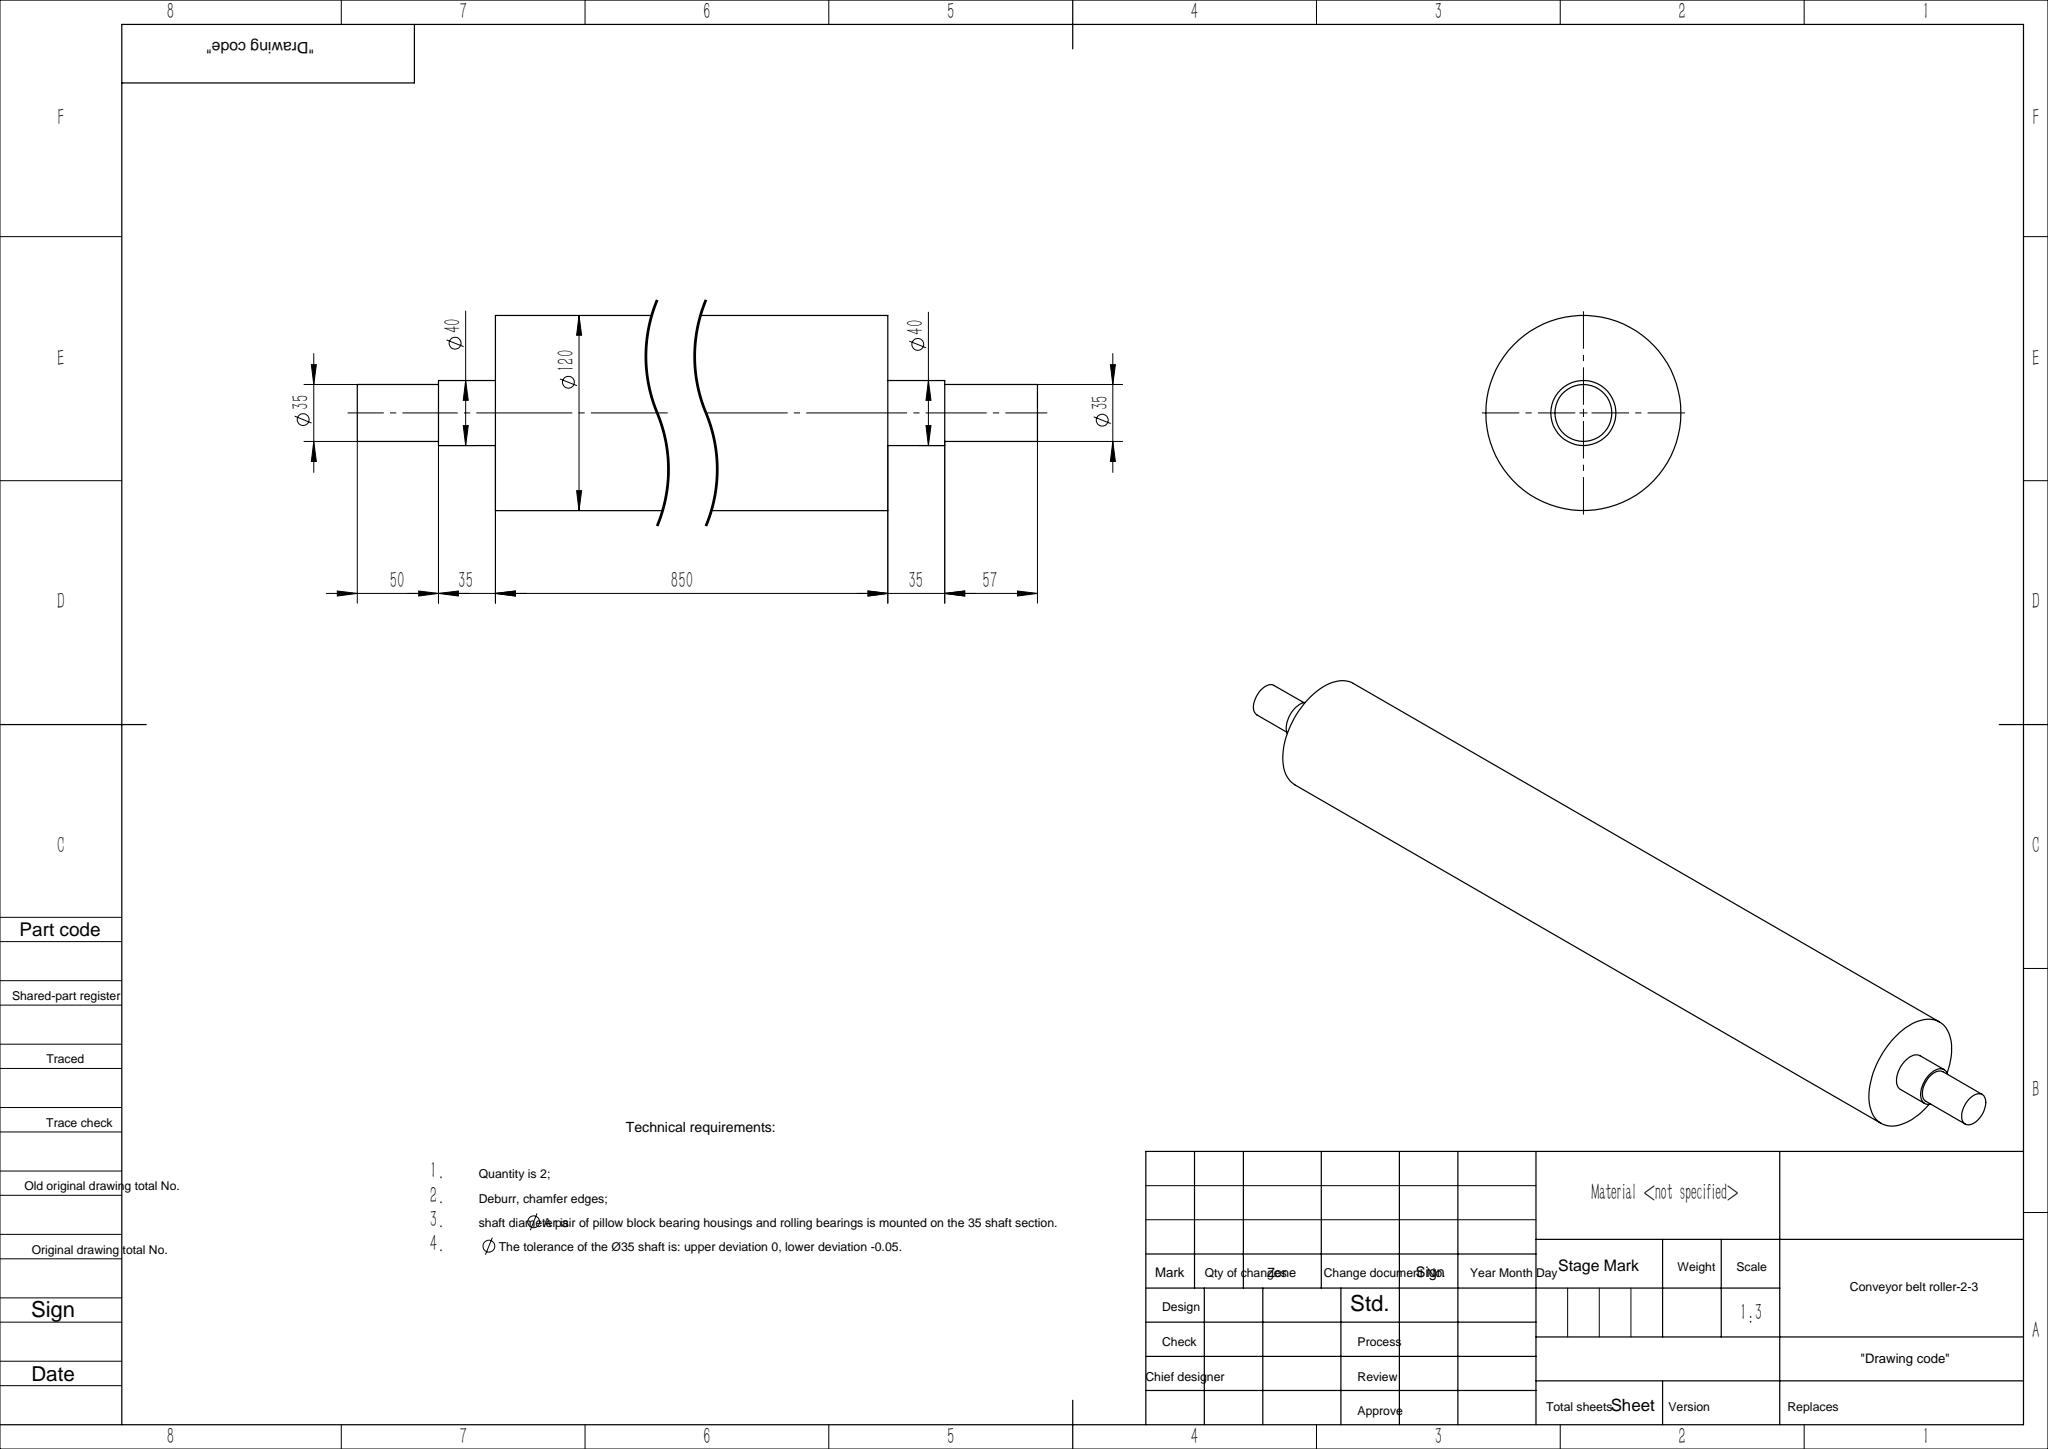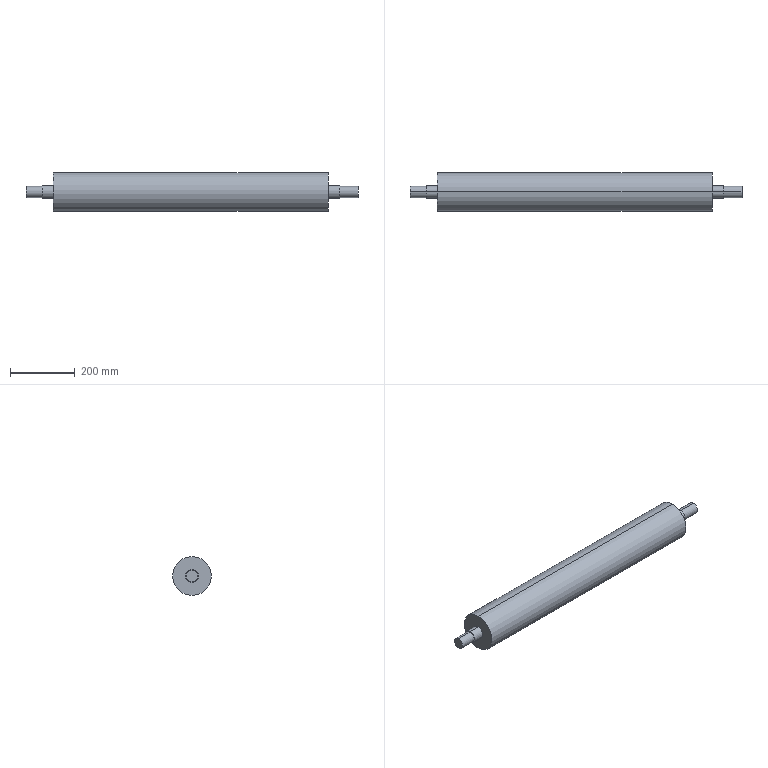Part | SolidWorks | features Revolution 1 | 1 solid | 16 faces | box 1027 x 120 x 120 mm | volume 9804184 mm3 | cylinder 10 | plane 6 | commonest cylinder face diameters 35 x4 40 x4 120 x2
STEP:
#1=CARTESIAN_POINT('',(970.,0.,-17.5));
#2=VERTEX_POINT('',#1);
#3=CARTESIAN_POINT('',(970.,0.,17.5));
#4=VERTEX_POINT('',#3);
#5=CARTESIAN_POINT('',(970.,0.,0.));
#6=DIRECTION('',(1.,0.,0.));
#7=DIRECTION('',(0.,0.,-1.));
#8=AXIS2_PLACEMENT_3D('',#5,#6,#7);
#9=CIRCLE('',#8,17.5);
#10=EDGE_CURVE('',#2,#4,#9,.T.);
#11=ORIENTED_EDGE('',*,*,#10,.T.);
#12=CARTESIAN_POINT('',(1027.,0.,17.5));
#13=VERTEX_POINT('',#12);
#14=CARTESIAN_POINT('',(1027.,0.,17.5));
#15=DIRECTION('',(1.,0.,0.));
#16=VECTOR('',#15,1000.);
#17=LINE('',#14,#16);
#18=EDGE_CURVE('',#4,#13,#17,.T.);
#19=ORIENTED_EDGE('',*,*,#18,.T.);
#20=CARTESIAN_POINT('',(1027.,0.,-17.5));
#21=VERTEX_POINT('',#20);
#22=CARTESIAN_POINT('',(1027.,0.,0.));
#23=DIRECTION('',(1.,0.,0.));
#24=DIRECTION('',(0.,0.,-1.));
#25=AXIS2_PLACEMENT_3D('',#22,#23,#24);
#26=CIRCLE('',#25,17.5);
#27=EDGE_CURVE('',#21,#13,#26,.T.);
#28=ORIENTED_EDGE('',*,*,#27,.F.);
#29=CARTESIAN_POINT('',(1027.,0.,-17.5));
#30=DIRECTION('',(1.,0.,0.));
#31=VECTOR('',#30,1000.);
#32=LINE('',#29,#31);
#33=EDGE_CURVE('',#2,#21,#32,.T.);
#34=ORIENTED_EDGE('',*,*,#33,.F.);
#35=EDGE_LOOP('',(#11,#19,#28,#34));
#36=FACE_OUTER_BOUND('',#35,.T.);
#37=CARTESIAN_POINT('',(1027.,0.,0.));
#38=DIRECTION('',(1.,0.,0.));
#39=DIRECTION('',(0.,0.,-1.));
#40=AXIS2_PLACEMENT_3D('',#37,#38,#39);
#41=CYLINDRICAL_SURFACE('',#40,17.5);
#42=ADVANCED_FACE('',(#36),#41,.T.);
#43=CARTESIAN_POINT('',(935.,0.,-20.));
#44=VERTEX_POINT('',#43);
#45=CARTESIAN_POINT('',(935.,0.,20.));
#46=VERTEX_POINT('',#45);
#47=CARTESIAN_POINT('',(935.,0.,0.));
#48=DIRECTION('',(1.,0.,0.));
#49=DIRECTION('',(0.,0.,-1.));
#50=AXIS2_PLACEMENT_3D('',#47,#48,#49);
#51=CIRCLE('',#50,20.);
#52=EDGE_CURVE('',#44,#46,#51,.T.);
#53=ORIENTED_EDGE('',*,*,#52,.T.);
#54=CARTESIAN_POINT('',(970.,0.,20.));
#55=VERTEX_POINT('',#54);
#56=CARTESIAN_POINT('',(1027.,0.,20.));
#57=DIRECTION('',(1.,0.,0.));
#58=VECTOR('',#57,1000.);
#59=LINE('',#56,#58);
#60=EDGE_CURVE('',#46,#55,#59,.T.);
#61=ORIENTED_EDGE('',*,*,#60,.T.);
#62=CARTESIAN_POINT('',(970.,0.,-20.));
#63=VERTEX_POINT('',#62);
#64=CARTESIAN_POINT('',(970.,0.,0.));
#65=DIRECTION('',(1.,0.,0.));
#66=DIRECTION('',(0.,0.,-1.));
#67=AXIS2_PLACEMENT_3D('',#64,#65,#66);
#68=CIRCLE('',#67,20.);
#69=EDGE_CURVE('',#63,#55,#68,.T.);
#70=ORIENTED_EDGE('',*,*,#69,.F.);
#71=CARTESIAN_POINT('',(1027.,0.,-20.));
#72=DIRECTION('',(1.,0.,0.));
#73=VECTOR('',#72,1000.);
#74=LINE('',#71,#73);
#75=EDGE_CURVE('',#44,#63,#74,.T.);
#76=ORIENTED_EDGE('',*,*,#75,.F.);
#77=EDGE_LOOP('',(#53,#61,#70,#76));
#78=FACE_OUTER_BOUND('',#77,.T.);
#79=CARTESIAN_POINT('',(1027.,0.,0.));
#80=DIRECTION('',(1.,0.,0.));
#81=DIRECTION('',(0.,0.,-1.));
#82=AXIS2_PLACEMENT_3D('',#79,#80,#81);
#83=CYLINDRICAL_SURFACE('',#82,20.);
#84=ADVANCED_FACE('',(#78),#83,.T.);
#85=CARTESIAN_POINT('',(85.,0.,-60.));
#86=VERTEX_POINT('',#85);
#87=CARTESIAN_POINT('',(85.,0.,60.));
#88=VERTEX_POINT('',#87);
#89=CARTESIAN_POINT('',(85.,0.,0.));
#90=DIRECTION('',(1.,0.,0.));
#91=DIRECTION('',(0.,0.,-1.));
#92=AXIS2_PLACEMENT_3D('',#89,#90,#91);
#93=CIRCLE('',#92,60.);
#94=EDGE_CURVE('',#86,#88,#93,.T.);
#95=ORIENTED_EDGE('',*,*,#94,.T.);
#96=CARTESIAN_POINT('',(935.,0.,60.));
#97=VERTEX_POINT('',#96);
#98=CARTESIAN_POINT('',(1027.,0.,60.));
#99=DIRECTION('',(1.,0.,0.));
#100=VECTOR('',#99,1000.);
#101=LINE('',#98,#100);
#102=EDGE_CURVE('',#88,#97,#101,.T.);
#103=ORIENTED_EDGE('',*,*,#102,.T.);
#104=CARTESIAN_POINT('',(935.,0.,-60.));
#105=VERTEX_POINT('',#104);
#106=CARTESIAN_POINT('',(935.,0.,0.));
#107=DIRECTION('',(1.,0.,0.));
#108=DIRECTION('',(0.,0.,-1.));
#109=AXIS2_PLACEMENT_3D('',#106,#107,#108);
#110=CIRCLE('',#109,60.);
#111=EDGE_CURVE('',#105,#97,#110,.T.);
#112=ORIENTED_EDGE('',*,*,#111,.F.);
#113=CARTESIAN_POINT('',(1027.,0.,-60.));
#114=DIRECTION('',(1.,0.,0.));
#115=VECTOR('',#114,1000.);
#116=LINE('',#113,#115);
#117=EDGE_CURVE('',#86,#105,#116,.T.);
#118=ORIENTED_EDGE('',*,*,#117,.F.);
#119=EDGE_LOOP('',(#95,#103,#112,#118));
#120=FACE_OUTER_BOUND('',#119,.T.);
#121=CARTESIAN_POINT('',(1027.,0.,0.));
#122=DIRECTION('',(1.,0.,0.));
#123=DIRECTION('',(0.,0.,-1.));
#124=AXIS2_PLACEMENT_3D('',#121,#122,#123);
#125=CYLINDRICAL_SURFACE('',#124,60.);
#126=ADVANCED_FACE('',(#120),#125,.T.);
#127=CARTESIAN_POINT('',(50.,0.,-20.));
#128=VERTEX_POINT('',#127);
#129=CARTESIAN_POINT('',(50.,0.,20.));
#130=VERTEX_POINT('',#129);
#131=CARTESIAN_POINT('',(50.,0.,0.));
#132=DIRECTION('',(1.,0.,0.));
#133=DIRECTION('',(0.,0.,-1.));
#134=AXIS2_PLACEMENT_3D('',#131,#132,#133);
#135=CIRCLE('',#134,20.);
#136=EDGE_CURVE('',#128,#130,#135,.T.);
#137=ORIENTED_EDGE('',*,*,#136,.T.);
#138=CARTESIAN_POINT('',(85.,0.,20.));
#139=VERTEX_POINT('',#138);
#140=CARTESIAN_POINT('',(1027.,0.,20.));
#141=DIRECTION('',(1.,0.,0.));
#142=VECTOR('',#141,1000.);
#143=LINE('',#140,#142);
#144=EDGE_CURVE('',#130,#139,#143,.T.);
#145=ORIENTED_EDGE('',*,*,#144,.T.);
#146=CARTESIAN_POINT('',(85.,0.,-20.));
#147=VERTEX_POINT('',#146);
#148=CARTESIAN_POINT('',(85.,0.,0.));
#149=DIRECTION('',(1.,0.,0.));
#150=DIRECTION('',(0.,0.,-1.));
#151=AXIS2_PLACEMENT_3D('',#148,#149,#150);
#152=CIRCLE('',#151,20.);
#153=EDGE_CURVE('',#147,#139,#152,.T.);
#154=ORIENTED_EDGE('',*,*,#153,.F.);
#155=CARTESIAN_POINT('',(1027.,0.,-20.));
#156=DIRECTION('',(1.,0.,0.));
#157=VECTOR('',#156,1000.);
#158=LINE('',#155,#157);
#159=EDGE_CURVE('',#128,#147,#158,.T.);
#160=ORIENTED_EDGE('',*,*,#159,.F.);
#161=EDGE_LOOP('',(#137,#145,#154,#160));
#162=FACE_OUTER_BOUND('',#161,.T.);
#163=CARTESIAN_POINT('',(1027.,0.,0.));
#164=DIRECTION('',(1.,0.,0.));
#165=DIRECTION('',(0.,0.,-1.));
#166=AXIS2_PLACEMENT_3D('',#163,#164,#165);
#167=CYLINDRICAL_SURFACE('',#166,20.);
#168=ADVANCED_FACE('',(#162),#167,.T.);
#169=CARTESIAN_POINT('',(0.,0.,-17.5));
#170=VERTEX_POINT('',#169);
#171=CARTESIAN_POINT('',(0.,0.,17.5));
#172=VERTEX_POINT('',#171);
#173=CARTESIAN_POINT('',(0.,0.,0.));
#174=DIRECTION('',(1.,0.,0.));
#175=DIRECTION('',(0.,0.,-1.));
#176=AXIS2_PLACEMENT_3D('',#173,#174,#175);
#177=CIRCLE('',#176,17.5);
#178=EDGE_CURVE('',#170,#172,#177,.T.);
#179=ORIENTED_EDGE('',*,*,#178,.T.);
#180=CARTESIAN_POINT('',(50.,0.,17.5));
#181=VERTEX_POINT('',#180);
#182=CARTESIAN_POINT('',(1027.,0.,17.5));
#183=DIRECTION('',(1.,0.,0.));
#184=VECTOR('',#183,1000.);
#185=LINE('',#182,#184);
#186=EDGE_CURVE('',#172,#181,#185,.T.);
#187=ORIENTED_EDGE('',*,*,#186,.T.);
#188=CARTESIAN_POINT('',(50.,0.,-17.5));
#189=VERTEX_POINT('',#188);
#190=CARTESIAN_POINT('',(50.,0.,0.));
#191=DIRECTION('',(1.,0.,0.));
#192=DIRECTION('',(0.,0.,-1.));
#193=AXIS2_PLACEMENT_3D('',#190,#191,#192);
#194=CIRCLE('',#193,17.5);
#195=EDGE_CURVE('',#189,#181,#194,.T.);
#196=ORIENTED_EDGE('',*,*,#195,.F.);
#197=CARTESIAN_POINT('',(1027.,0.,-17.5));
#198=DIRECTION('',(1.,0.,0.));
#199=VECTOR('',#198,1000.);
#200=LINE('',#197,#199);
#201=EDGE_CURVE('',#170,#189,#200,.T.);
#202=ORIENTED_EDGE('',*,*,#201,.F.);
#203=EDGE_LOOP('',(#179,#187,#196,#202));
#204=FACE_OUTER_BOUND('',#203,.T.);
#205=CARTESIAN_POINT('',(1027.,0.,0.));
#206=DIRECTION('',(1.,0.,0.));
#207=DIRECTION('',(0.,0.,-1.));
#208=AXIS2_PLACEMENT_3D('',#205,#206,#207);
#209=CYLINDRICAL_SURFACE('',#208,17.5);
#210=ADVANCED_FACE('',(#204),#209,.T.);
#211=ORIENTED_EDGE('',*,*,#178,.F.);
#212=CARTESIAN_POINT('',(0.,0.,0.));
#213=DIRECTION('',(1.,0.,0.));
#214=DIRECTION('',(0.,0.,-1.));
#215=AXIS2_PLACEMENT_3D('',#212,#213,#214);
#216=CIRCLE('',#215,17.5);
#217=EDGE_CURVE('',#172,#170,#216,.T.);
#218=ORIENTED_EDGE('',*,*,#217,.F.);
#219=EDGE_LOOP('',(#211,#218));
#220=FACE_OUTER_BOUND('',#219,.T.);
#221=CARTESIAN_POINT('',(0.,0.,0.));
#222=DIRECTION('',(-1.,0.,0.));
#223=DIRECTION('',(0.,0.,1.));
#224=AXIS2_PLACEMENT_3D('',#221,#222,#223);
#225=PLANE('',#224);
#226=ADVANCED_FACE('',(#220),#225,.T.);
#227=ORIENTED_EDGE('',*,*,#186,.F.);
#228=ORIENTED_EDGE('',*,*,#217,.T.);
#229=ORIENTED_EDGE('',*,*,#201,.T.);
#230=CARTESIAN_POINT('',(50.,0.,0.));
#231=DIRECTION('',(1.,0.,0.));
#232=DIRECTION('',(0.,0.,-1.));
#233=AXIS2_PLACEMENT_3D('',#230,#231,#232);
#234=CIRCLE('',#233,17.5);
#235=EDGE_CURVE('',#181,#189,#234,.T.);
#236=ORIENTED_EDGE('',*,*,#235,.F.);
#237=EDGE_LOOP('',(#227,#228,#229,#236));
#238=FACE_OUTER_BOUND('',#237,.T.);
#239=CARTESIAN_POINT('',(1027.,0.,0.));
#240=DIRECTION('',(1.,0.,0.));
#241=DIRECTION('',(0.,0.,-1.));
#242=AXIS2_PLACEMENT_3D('',#239,#240,#241);
#243=CYLINDRICAL_SURFACE('',#242,17.5);
#244=ADVANCED_FACE('',(#238),#243,.T.);
#245=ORIENTED_EDGE('',*,*,#195,.T.);
#246=ORIENTED_EDGE('',*,*,#235,.T.);
#247=EDGE_LOOP('',(#245,#246));
#248=FACE_BOUND('',#247,.T.);
#249=ORIENTED_EDGE('',*,*,#136,.F.);
#250=CARTESIAN_POINT('',(50.,0.,0.));
#251=DIRECTION('',(1.,0.,0.));
#252=DIRECTION('',(0.,0.,-1.));
#253=AXIS2_PLACEMENT_3D('',#250,#251,#252);
#254=CIRCLE('',#253,20.);
#255=EDGE_CURVE('',#130,#128,#254,.T.);
#256=ORIENTED_EDGE('',*,*,#255,.F.);
#257=EDGE_LOOP('',(#249,#256));
#258=FACE_OUTER_BOUND('',#257,.T.);
#259=CARTESIAN_POINT('',(50.,17.5,0.));
#260=DIRECTION('',(-1.,0.,0.));
#261=DIRECTION('',(0.,0.,1.));
#262=AXIS2_PLACEMENT_3D('',#259,#260,#261);
#263=PLANE('',#262);
#264=ADVANCED_FACE('',(#248,#258),#263,.T.);
#265=ORIENTED_EDGE('',*,*,#144,.F.);
#266=ORIENTED_EDGE('',*,*,#255,.T.);
#267=ORIENTED_EDGE('',*,*,#159,.T.);
#268=CARTESIAN_POINT('',(85.,0.,0.));
#269=DIRECTION('',(1.,0.,0.));
#270=DIRECTION('',(0.,0.,-1.));
#271=AXIS2_PLACEMENT_3D('',#268,#269,#270);
#272=CIRCLE('',#271,20.);
#273=EDGE_CURVE('',#139,#147,#272,.T.);
#274=ORIENTED_EDGE('',*,*,#273,.F.);
#275=EDGE_LOOP('',(#265,#266,#267,#274));
#276=FACE_OUTER_BOUND('',#275,.T.);
#277=CARTESIAN_POINT('',(1027.,0.,0.));
#278=DIRECTION('',(1.,0.,0.));
#279=DIRECTION('',(0.,0.,-1.));
#280=AXIS2_PLACEMENT_3D('',#277,#278,#279);
#281=CYLINDRICAL_SURFACE('',#280,20.);
#282=ADVANCED_FACE('',(#276),#281,.T.);
#283=ORIENTED_EDGE('',*,*,#153,.T.);
#284=ORIENTED_EDGE('',*,*,#273,.T.);
#285=EDGE_LOOP('',(#283,#284));
#286=FACE_BOUND('',#285,.T.);
#287=ORIENTED_EDGE('',*,*,#94,.F.);
#288=CARTESIAN_POINT('',(85.,0.,0.));
#289=DIRECTION('',(1.,0.,0.));
#290=DIRECTION('',(0.,0.,-1.));
#291=AXIS2_PLACEMENT_3D('',#288,#289,#290);
#292=CIRCLE('',#291,60.);
#293=EDGE_CURVE('',#88,#86,#292,.T.);
#294=ORIENTED_EDGE('',*,*,#293,.F.);
#295=EDGE_LOOP('',(#287,#294));
#296=FACE_OUTER_BOUND('',#295,.T.);
#297=CARTESIAN_POINT('',(85.,20.,0.));
#298=DIRECTION('',(-1.,0.,0.));
#299=DIRECTION('',(0.,0.,1.));
#300=AXIS2_PLACEMENT_3D('',#297,#298,#299);
#301=PLANE('',#300);
#302=ADVANCED_FACE('',(#286,#296),#301,.T.);
#303=ORIENTED_EDGE('',*,*,#102,.F.);
#304=ORIENTED_EDGE('',*,*,#293,.T.);
#305=ORIENTED_EDGE('',*,*,#117,.T.);
#306=CARTESIAN_POINT('',(935.,0.,0.));
#307=DIRECTION('',(1.,0.,0.));
#308=DIRECTION('',(0.,0.,-1.));
#309=AXIS2_PLACEMENT_3D('',#306,#307,#308);
#310=CIRCLE('',#309,60.);
#311=EDGE_CURVE('',#97,#105,#310,.T.);
#312=ORIENTED_EDGE('',*,*,#311,.F.);
#313=EDGE_LOOP('',(#303,#304,#305,#312));
#314=FACE_OUTER_BOUND('',#313,.T.);
#315=CARTESIAN_POINT('',(1027.,0.,0.));
#316=DIRECTION('',(1.,0.,0.));
#317=DIRECTION('',(0.,0.,-1.));
#318=AXIS2_PLACEMENT_3D('',#315,#316,#317);
#319=CYLINDRICAL_SURFACE('',#318,60.);
#320=ADVANCED_FACE('',(#314),#319,.T.);
#321=ORIENTED_EDGE('',*,*,#111,.T.);
#322=ORIENTED_EDGE('',*,*,#311,.T.);
#323=EDGE_LOOP('',(#321,#322));
#324=FACE_OUTER_BOUND('',#323,.T.);
#325=ORIENTED_EDGE('',*,*,#52,.F.);
#326=CARTESIAN_POINT('',(935.,0.,0.));
#327=DIRECTION('',(1.,0.,0.));
#328=DIRECTION('',(0.,0.,-1.));
#329=AXIS2_PLACEMENT_3D('',#326,#327,#328);
#330=CIRCLE('',#329,20.);
#331=EDGE_CURVE('',#46,#44,#330,.T.);
#332=ORIENTED_EDGE('',*,*,#331,.F.);
#333=EDGE_LOOP('',(#325,#332));
#334=FACE_BOUND('',#333,.T.);
#335=CARTESIAN_POINT('',(935.,60.,0.));
#336=DIRECTION('',(1.,0.,0.));
#337=DIRECTION('',(0.,0.,-1.));
#338=AXIS2_PLACEMENT_3D('',#335,#336,#337);
#339=PLANE('',#338);
#340=ADVANCED_FACE('',(#324,#334),#339,.T.);
#341=ORIENTED_EDGE('',*,*,#60,.F.);
#342=ORIENTED_EDGE('',*,*,#331,.T.);
#343=ORIENTED_EDGE('',*,*,#75,.T.);
#344=CARTESIAN_POINT('',(970.,0.,0.));
#345=DIRECTION('',(1.,0.,0.));
#346=DIRECTION('',(0.,0.,-1.));
#347=AXIS2_PLACEMENT_3D('',#344,#345,#346);
#348=CIRCLE('',#347,20.);
#349=EDGE_CURVE('',#55,#63,#348,.T.);
#350=ORIENTED_EDGE('',*,*,#349,.F.);
#351=EDGE_LOOP('',(#341,#342,#343,#350));
#352=FACE_OUTER_BOUND('',#351,.T.);
#353=CARTESIAN_POINT('',(1027.,0.,0.));
#354=DIRECTION('',(1.,0.,0.));
#355=DIRECTION('',(0.,0.,-1.));
#356=AXIS2_PLACEMENT_3D('',#353,#354,#355);
#357=CYLINDRICAL_SURFACE('',#356,20.);
#358=ADVANCED_FACE('',(#352),#357,.T.);
#359=ORIENTED_EDGE('',*,*,#69,.T.);
#360=ORIENTED_EDGE('',*,*,#349,.T.);
#361=EDGE_LOOP('',(#359,#360));
#362=FACE_OUTER_BOUND('',#361,.T.);
#363=ORIENTED_EDGE('',*,*,#10,.F.);
#364=CARTESIAN_POINT('',(970.,0.,0.));
#365=DIRECTION('',(1.,0.,0.));
#366=DIRECTION('',(0.,0.,-1.));
#367=AXIS2_PLACEMENT_3D('',#364,#365,#366);
#368=CIRCLE('',#367,17.5);
#369=EDGE_CURVE('',#4,#2,#368,.T.);
#370=ORIENTED_EDGE('',*,*,#369,.F.);
#371=EDGE_LOOP('',(#363,#370));
#372=FACE_BOUND('',#371,.T.);
#373=CARTESIAN_POINT('',(970.,20.,0.));
#374=DIRECTION('',(1.,0.,0.));
#375=DIRECTION('',(0.,0.,-1.));
#376=AXIS2_PLACEMENT_3D('',#373,#374,#375);
#377=PLANE('',#376);
#378=ADVANCED_FACE('',(#362,#372),#377,.T.);
#379=ORIENTED_EDGE('',*,*,#18,.F.);
#380=ORIENTED_EDGE('',*,*,#369,.T.);
#381=ORIENTED_EDGE('',*,*,#33,.T.);
#382=CARTESIAN_POINT('',(1027.,0.,0.));
#383=DIRECTION('',(1.,0.,0.));
#384=DIRECTION('',(0.,0.,-1.));
#385=AXIS2_PLACEMENT_3D('',#382,#383,#384);
#386=CIRCLE('',#385,17.5);
#387=EDGE_CURVE('',#13,#21,#386,.T.);
#388=ORIENTED_EDGE('',*,*,#387,.F.);
#389=EDGE_LOOP('',(#379,#380,#381,#388));
#390=FACE_OUTER_BOUND('',#389,.T.);
#391=CARTESIAN_POINT('',(1027.,0.,0.));
#392=DIRECTION('',(1.,0.,0.));
#393=DIRECTION('',(0.,0.,-1.));
#394=AXIS2_PLACEMENT_3D('',#391,#392,#393);
#395=CYLINDRICAL_SURFACE('',#394,17.5);
#396=ADVANCED_FACE('',(#390),#395,.T.);
#397=ORIENTED_EDGE('',*,*,#27,.T.);
#398=ORIENTED_EDGE('',*,*,#387,.T.);
#399=EDGE_LOOP('',(#397,#398));
#400=FACE_OUTER_BOUND('',#399,.T.);
#401=CARTESIAN_POINT('',(1027.,17.5,0.));
#402=DIRECTION('',(1.,0.,0.));
#403=DIRECTION('',(0.,0.,-1.));
#404=AXIS2_PLACEMENT_3D('',#401,#402,#403);
#405=PLANE('',#404);
#406=ADVANCED_FACE('',(#400),#405,.T.);
#407=CLOSED_SHELL('',(#42,#84,#126,#168,#210,#226,#244,#264,#282,#302,#320,#340,#358,#378,#396,#406));
#408=MANIFOLD_SOLID_BREP('',#407);
#409=CARTESIAN_POINT('',(0.,0.,0.));
#410=DIRECTION('',(0.,0.,1.));
#411=DIRECTION('',(1.,0.,0.));
#412=AXIS2_PLACEMENT_3D('',#409,#410,#411);
#413=(LENGTH_UNIT()NAMED_UNIT(*)SI_UNIT(.MILLI.,.METRE.));
#414=UNCERTAINTY_MEASURE_WITH_UNIT(LENGTH_MEASURE(0.00001),#413,'','');
#415=(NAMED_UNIT(*)PLANE_ANGLE_UNIT()SI_UNIT($,.RADIAN.));
#416=(NAMED_UNIT(*)SI_UNIT($,.STERADIAN.)SOLID_ANGLE_UNIT());
#417=(GEOMETRIC_REPRESENTATION_CONTEXT(3)GLOBAL_UNCERTAINTY_ASSIGNED_CONTEXT((#414))GLOBAL_UNIT_ASSIGNED_CONTEXT((#413,#415,#416))REPRESENTATION_CONTEXT('',''));
#418=ADVANCED_BREP_SHAPE_REPRESENTATION('',(#408,#412),#417);